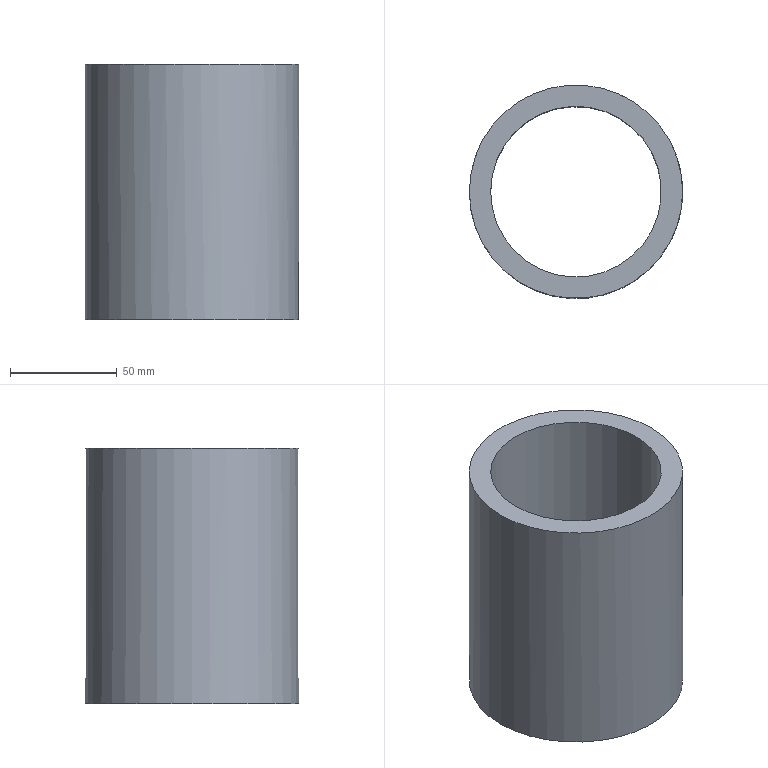Part | NX | features solid 2 | 1 solid | 6 faces | box 100 x 100 x 120 mm | volume 338292 mm3 | cylinder 3 | plane 2 | cone 1 | commonest cylinder face diameters 10 x1 80 x1 100 x1
STEP:
#1=CARTESIAN_POINT('',(1395.,-495.,-205.));
#2=VERTEX_POINT('',#1);
#3=CARTESIAN_POINT('',(1445.,-495.,-205.));
#4=DIRECTION('',(0.,0.,-1.));
#5=DIRECTION('',(-1.,0.,0.));
#6=AXIS2_PLACEMENT_3D('',#3,#4,#5);
#7=CIRCLE('',#6,50.);
#8=EDGE_CURVE('',#2,#2,#7,.T.);
#9=ORIENTED_EDGE('',*,*,#8,.T.);
#10=EDGE_LOOP('',(#9));
#11=FACE_BOUND('',#10,.T.);
#12=CARTESIAN_POINT('',(1494.75,-499.994,-300.));
#13=VERTEX_POINT('',#12);
#14=CARTESIAN_POINT('',(1494.75,-499.994,-325.));
#15=VERTEX_POINT('',#14);
#16=CARTESIAN_POINT('',(1494.75,-499.994,-315.));
#17=DIRECTION('',(0.,0.,-1.));
#18=VECTOR('',#17,1000.);
#19=LINE('',#16,#18);
#20=EDGE_CURVE('',#13,#15,#19,.T.);
#21=ORIENTED_EDGE('',*,*,#20,.F.);
#22=CARTESIAN_POINT('',(1495.,-495.,-296.996));
#23=VERTEX_POINT('',#22);
#24=CARTESIAN_POINT('',(1495.,-495.,-296.996));
#25=CARTESIAN_POINT('',(1495.,-496.668,-297.998));
#26=CARTESIAN_POINT('',(1494.916,-498.336,-299.));
#27=CARTESIAN_POINT('',(1494.75,-499.994,-300.));
#28=B_SPLINE_CURVE_WITH_KNOTS('',3,(#24,#25,#26,#27),.UNSPECIFIED.,.F.,.F.,(4,4),(-0.000000022,0.005837),.UNSPECIFIED.);
#29=EDGE_CURVE('',#13,#23,#28,.F.);
#30=ORIENTED_EDGE('',*,*,#29,.T.);
#31=CARTESIAN_POINT('',(1494.75,-490.006,-300.));
#32=VERTEX_POINT('',#31);
#33=CARTESIAN_POINT('',(1495.,-495.,-296.996));
#34=CARTESIAN_POINT('',(1495.,-493.332,-297.998));
#35=CARTESIAN_POINT('',(1494.916,-491.664,-299.));
#36=CARTESIAN_POINT('',(1494.75,-490.006,-300.));
#37=B_SPLINE_CURVE_WITH_KNOTS('',3,(#33,#34,#35,#36),.UNSPECIFIED.,.F.,.F.,(4,4),(-0.000000022,0.005837),.UNSPECIFIED.);
#38=EDGE_CURVE('',#23,#32,#37,.T.);
#39=ORIENTED_EDGE('',*,*,#38,.T.);
#40=CARTESIAN_POINT('',(1494.75,-490.006,-325.));
#41=VERTEX_POINT('',#40);
#42=CARTESIAN_POINT('',(1494.75,-490.006,-315.));
#43=DIRECTION('',(0.,0.,-1.));
#44=VECTOR('',#43,1000.);
#45=LINE('',#42,#44);
#46=EDGE_CURVE('',#41,#32,#45,.F.);
#47=ORIENTED_EDGE('',*,*,#46,.F.);
#48=CARTESIAN_POINT('',(1445.,-495.,-325.));
#49=DIRECTION('',(0.,0.,-1.));
#50=DIRECTION('',(-1.,0.,0.));
#51=AXIS2_PLACEMENT_3D('',#48,#49,#50);
#52=CIRCLE('',#51,50.);
#53=EDGE_CURVE('',#15,#41,#52,.T.);
#54=ORIENTED_EDGE('',*,*,#53,.F.);
#55=EDGE_LOOP('',(#21,#30,#39,#47,#54));
#56=FACE_BOUND('',#55,.T.);
#57=CARTESIAN_POINT('',(1445.,-495.,-205.));
#58=DIRECTION('',(0.,0.,-1.));
#59=DIRECTION('',(1.,0.,0.));
#60=AXIS2_PLACEMENT_3D('',#57,#58,#59);
#61=CYLINDRICAL_SURFACE('',#60,50.);
#62=ADVANCED_FACE('',(#11,#56),#61,.T.);
#63=CARTESIAN_POINT('',(1405.,-495.,-325.));
#64=VERTEX_POINT('',#63);
#65=CARTESIAN_POINT('',(1445.,-495.,-325.));
#66=DIRECTION('',(0.,0.,-1.));
#67=DIRECTION('',(-1.,0.,0.));
#68=AXIS2_PLACEMENT_3D('',#65,#66,#67);
#69=CIRCLE('',#68,40.);
#70=EDGE_CURVE('',#64,#64,#69,.T.);
#71=ORIENTED_EDGE('',*,*,#70,.F.);
#72=EDGE_LOOP('',(#71));
#73=FACE_BOUND('',#72,.T.);
#74=CARTESIAN_POINT('',(1495.,-495.,-325.));
#75=DIRECTION('',(0.,0.,-1.));
#76=DIRECTION('',(-1.,0.,0.));
#77=AXIS2_PLACEMENT_3D('',#74,#75,#76);
#78=CIRCLE('',#77,5.);
#79=EDGE_CURVE('',#41,#15,#78,.F.);
#80=ORIENTED_EDGE('',*,*,#79,.T.);
#81=ORIENTED_EDGE('',*,*,#53,.T.);
#82=EDGE_LOOP('',(#80,#81));
#83=FACE_BOUND('',#82,.T.);
#84=CARTESIAN_POINT('',(1445.,-495.,-325.));
#85=DIRECTION('',(0.,0.,1.));
#86=DIRECTION('',(-1.,0.,0.));
#87=AXIS2_PLACEMENT_3D('',#84,#85,#86);
#88=PLANE('',#87);
#89=ADVANCED_FACE('',(#73,#83),#88,.F.);
#90=CARTESIAN_POINT('',(1405.,-495.,-205.));
#91=VERTEX_POINT('',#90);
#92=CARTESIAN_POINT('',(1445.,-495.,-205.));
#93=DIRECTION('',(0.,0.,-1.));
#94=DIRECTION('',(-1.,0.,0.));
#95=AXIS2_PLACEMENT_3D('',#92,#93,#94);
#96=CIRCLE('',#95,40.);
#97=EDGE_CURVE('',#91,#91,#96,.T.);
#98=ORIENTED_EDGE('',*,*,#97,.F.);
#99=EDGE_LOOP('',(#98));
#100=FACE_BOUND('',#99,.T.);
#101=ORIENTED_EDGE('',*,*,#70,.T.);
#102=EDGE_LOOP('',(#101));
#103=FACE_BOUND('',#102,.T.);
#104=CARTESIAN_POINT('',(1445.,-495.,-205.));
#105=DIRECTION('',(0.,0.,-1.));
#106=DIRECTION('',(1.,0.,0.));
#107=AXIS2_PLACEMENT_3D('',#104,#105,#106);
#108=CYLINDRICAL_SURFACE('',#107,40.);
#109=ADVANCED_FACE('',(#100,#103),#108,.F.);
#110=ORIENTED_EDGE('',*,*,#97,.T.);
#111=EDGE_LOOP('',(#110));
#112=FACE_BOUND('',#111,.T.);
#113=ORIENTED_EDGE('',*,*,#8,.F.);
#114=EDGE_LOOP('',(#113));
#115=FACE_BOUND('',#114,.T.);
#116=CARTESIAN_POINT('',(1445.,-495.,-205.));
#117=DIRECTION('',(0.,0.,1.));
#118=DIRECTION('',(-1.,0.,0.));
#119=AXIS2_PLACEMENT_3D('',#116,#117,#118);
#120=PLANE('',#119);
#121=ADVANCED_FACE('',(#112,#115),#120,.T.);
#122=ORIENTED_EDGE('',*,*,#20,.T.);
#123=ORIENTED_EDGE('',*,*,#79,.F.);
#124=ORIENTED_EDGE('',*,*,#46,.T.);
#125=CARTESIAN_POINT('',(1495.,-495.,-300.));
#126=DIRECTION('',(0.,0.,1.));
#127=DIRECTION('',(1.,0.,0.));
#128=AXIS2_PLACEMENT_3D('',#125,#126,#127);
#129=CIRCLE('',#128,5.);
#130=EDGE_CURVE('',#32,#13,#129,.T.);
#131=ORIENTED_EDGE('',*,*,#130,.T.);
#132=EDGE_LOOP('',(#122,#123,#124,#131));
#133=FACE_BOUND('',#132,.T.);
#134=CARTESIAN_POINT('',(1495.,-495.,-309.));
#135=DIRECTION('',(0.,0.,-1.));
#136=DIRECTION('',(1.,0.,0.));
#137=AXIS2_PLACEMENT_3D('',#134,#135,#136);
#138=CYLINDRICAL_SURFACE('',#137,5.);
#139=ADVANCED_FACE('',(#133),#138,.F.);
#140=ORIENTED_EDGE('',*,*,#29,.F.);
#141=ORIENTED_EDGE('',*,*,#130,.F.);
#142=ORIENTED_EDGE('',*,*,#38,.F.);
#143=EDGE_LOOP('',(#140,#141,#142));
#144=FACE_BOUND('',#143,.T.);
#145=CARTESIAN_POINT('',(1495.,-495.,-300.));
#146=DIRECTION('',(0.,0.,-1.));
#147=DIRECTION('',(-1.,0.,0.));
#148=AXIS2_PLACEMENT_3D('',#145,#146,#147);
#149=CONICAL_SURFACE('',#148,5.,1.03);
#150=ADVANCED_FACE('',(#144),#149,.F.);
#151=CLOSED_SHELL('',(#62,#89,#109,#121,#139,#150));
#152=MANIFOLD_SOLID_BREP('',#151);
#153=(LENGTH_UNIT()NAMED_UNIT(*)SI_UNIT(.MILLI.,.METRE.));
#154=UNCERTAINTY_MEASURE_WITH_UNIT(LENGTH_MEASURE(0.0508),#153,'','');
#155=(NAMED_UNIT(*)PLANE_ANGLE_UNIT()SI_UNIT($,.RADIAN.));
#156=(NAMED_UNIT(*)SI_UNIT($,.STERADIAN.)SOLID_ANGLE_UNIT());
#157=(GEOMETRIC_REPRESENTATION_CONTEXT(3)GLOBAL_UNCERTAINTY_ASSIGNED_CONTEXT((#154))GLOBAL_UNIT_ASSIGNED_CONTEXT((#153,#155,#156))REPRESENTATION_CONTEXT('',''));
#158=ADVANCED_BREP_SHAPE_REPRESENTATION('',(#152),#157);